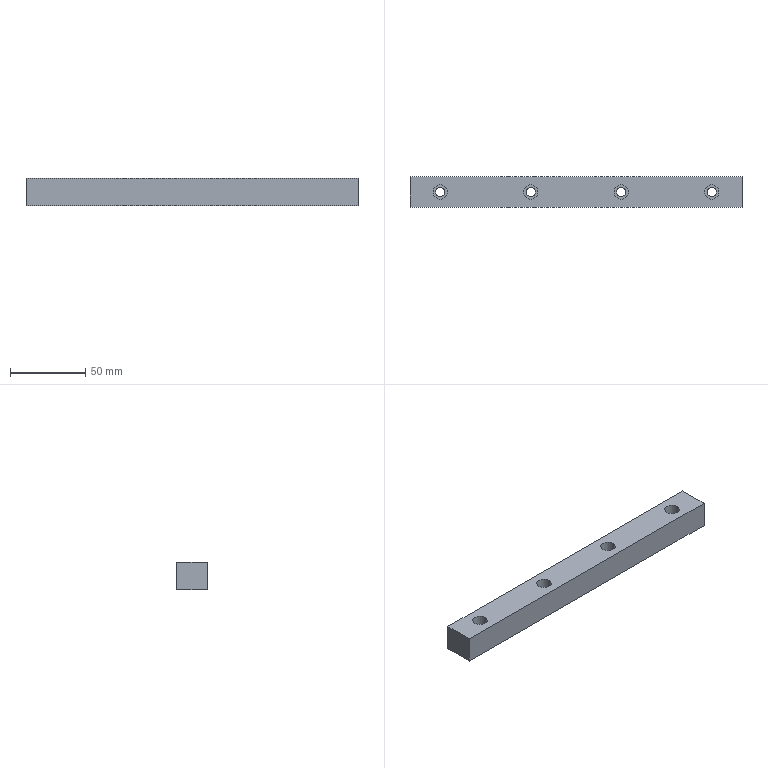Part | STEP file | MSA20LE slide rail | 1 solid | 26 faces | box 220 x 20 x 18 mm | volume 75716 mm3 | cylinder 16 | plane 10 | commonest cylinder face diameters 6 x8 9.5 x8